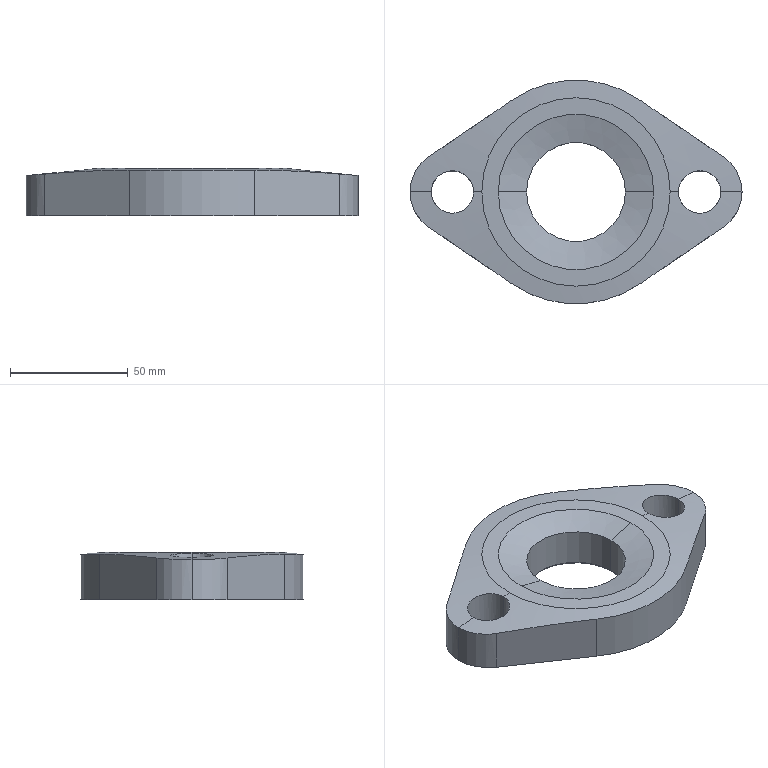Part | SolidWorks | features Chamfer 1, Extrusion 1, RevCut 1 | 1 solid | 23 faces | box 141 x 95 x 20 mm | volume 136049 mm3 | cylinder 11 | cone 6 | plane 6 | commonest cylinder face diameters 18 x4 36 x3 42 x2 95 x2
STEP:
#1=CARTESIAN_POINT('',(21.,0.,1.));
#2=VERTEX_POINT('',#1);
#3=CARTESIAN_POINT('',(-21.,0.,1.));
#4=VERTEX_POINT('',#3);
#5=CARTESIAN_POINT('',(0.,0.,1.));
#6=DIRECTION('',(0.,0.,-1.));
#7=DIRECTION('',(1.,0.,0.));
#8=AXIS2_PLACEMENT_3D('',#5,#6,#7);
#9=CIRCLE('',#8,21.);
#10=EDGE_CURVE('',#2,#4,#9,.T.);
#11=ORIENTED_EDGE('',*,*,#10,.F.);
#12=CARTESIAN_POINT('',(22.,0.,0.));
#13=VERTEX_POINT('',#12);
#14=CARTESIAN_POINT('',(21.,0.,1.));
#15=DIRECTION('',(0.7071,0.,-0.7071));
#16=VECTOR('',#15,1000.);
#17=LINE('',#14,#16);
#18=EDGE_CURVE('',#2,#13,#17,.T.);
#19=ORIENTED_EDGE('',*,*,#18,.T.);
#20=CARTESIAN_POINT('',(-22.,0.,0.));
#21=VERTEX_POINT('',#20);
#22=CARTESIAN_POINT('',(0.,0.,0.));
#23=DIRECTION('',(0.,0.,1.));
#24=DIRECTION('',(1.,0.,0.));
#25=AXIS2_PLACEMENT_3D('',#22,#23,#24);
#26=CIRCLE('',#25,22.);
#27=EDGE_CURVE('',#21,#13,#26,.T.);
#28=ORIENTED_EDGE('',*,*,#27,.F.);
#29=CARTESIAN_POINT('',(-21.,0.,1.));
#30=DIRECTION('',(-0.7071,0.,-0.7071));
#31=VECTOR('',#30,1000.);
#32=LINE('',#29,#31);
#33=EDGE_CURVE('',#4,#21,#32,.T.);
#34=ORIENTED_EDGE('',*,*,#33,.F.);
#35=EDGE_LOOP('',(#11,#19,#28,#34));
#36=FACE_OUTER_BOUND('',#35,.T.);
#37=CARTESIAN_POINT('',(0.,0.,1.));
#38=DIRECTION('',(0.,0.,-1.));
#39=DIRECTION('',(-1.,0.,0.));
#40=AXIS2_PLACEMENT_3D('',#37,#38,#39);
#41=CONICAL_SURFACE('',#40,21.,0.7854);
#42=ADVANCED_FACE('',(#36),#41,.F.);
#43=CARTESIAN_POINT('',(-40.,0.,20.));
#44=VERTEX_POINT('',#43);
#45=CARTESIAN_POINT('',(40.,0.,20.));
#46=VERTEX_POINT('',#45);
#47=CARTESIAN_POINT('',(0.,0.,20.));
#48=DIRECTION('',(0.,0.,-1.));
#49=DIRECTION('',(-1.,0.,0.));
#50=AXIS2_PLACEMENT_3D('',#47,#48,#49);
#51=CIRCLE('',#50,40.);
#52=EDGE_CURVE('',#44,#46,#51,.T.);
#53=ORIENTED_EDGE('',*,*,#52,.T.);
#54=CARTESIAN_POINT('',(43.5,0.,19.656));
#55=VERTEX_POINT('',#54);
#56=CARTESIAN_POINT('',(40.,0.,20.));
#57=DIRECTION('',(0.9952,0.,-0.09789));
#58=VECTOR('',#57,1000.);
#59=LINE('',#56,#58);
#60=EDGE_CURVE('',#46,#55,#59,.T.);
#61=ORIENTED_EDGE('',*,*,#60,.T.);
#62=CARTESIAN_POINT('',(61.5,0.,17.885));
#63=VERTEX_POINT('',#62);
#64=CARTESIAN_POINT('',(43.5,0.,19.656));
#65=CARTESIAN_POINT('',(43.5,0.5885,19.656));
#66=CARTESIAN_POINT('',(43.557,1.174,19.649));
#67=CARTESIAN_POINT('',(43.731,2.048,19.628));
#68=CARTESIAN_POINT('',(43.804,2.337,19.62));
#69=CARTESIAN_POINT('',(43.975,2.902,19.6));
#70=CARTESIAN_POINT('',(44.174,3.455,19.576));
#71=CARTESIAN_POINT('',(44.426,3.986,19.547));
#72=CARTESIAN_POINT('',(44.704,4.507,19.515));
#73=CARTESIAN_POINT('',(44.858,4.763,19.497));
#74=CARTESIAN_POINT('',(45.352,5.5,19.441));
#75=CARTESIAN_POINT('',(45.725,5.953,19.399));
#76=CARTESIAN_POINT('',(46.556,6.783,19.307));
#77=CARTESIAN_POINT('',(47.019,7.163,19.256));
#78=CARTESIAN_POINT('',(47.996,7.814,19.151));
#79=CARTESIAN_POINT('',(48.512,8.09,19.097));
#80=CARTESIAN_POINT('',(49.33,8.428,19.012));
#81=CARTESIAN_POINT('',(49.61,8.528,18.983));
#82=CARTESIAN_POINT('',(50.174,8.699,18.926));
#83=CARTESIAN_POINT('',(50.458,8.77,18.897));
#84=CARTESIAN_POINT('',(51.319,8.941,18.811));
#85=CARTESIAN_POINT('',(51.904,9.,18.753));
#86=CARTESIAN_POINT('',(53.089,9.,18.638));
#87=CARTESIAN_POINT('',(53.673,8.942,18.582));
#88=CARTESIAN_POINT('',(54.534,8.772,18.501));
#89=CARTESIAN_POINT('',(54.819,8.701,18.475));
#90=CARTESIAN_POINT('',(55.385,8.53,18.423));
#91=CARTESIAN_POINT('',(55.665,8.43,18.397));
#92=CARTESIAN_POINT('',(56.482,8.093,18.322));
#93=CARTESIAN_POINT('',(56.999,7.817,18.276));
#94=CARTESIAN_POINT('',(57.733,7.328,18.21));
#95=CARTESIAN_POINT('',(57.972,7.151,18.189));
#96=CARTESIAN_POINT('',(58.431,6.776,18.149));
#97=CARTESIAN_POINT('',(58.65,6.578,18.129));
#98=CARTESIAN_POINT('',(59.273,5.955,18.075));
#99=CARTESIAN_POINT('',(59.647,5.502,18.043));
#100=CARTESIAN_POINT('',(60.142,4.763,18.));
#101=CARTESIAN_POINT('',(60.296,4.507,17.987));
#102=CARTESIAN_POINT('',(60.574,3.987,17.963));
#103=CARTESIAN_POINT('',(60.826,3.456,17.942));
#104=CARTESIAN_POINT('',(61.024,2.902,17.925));
#105=CARTESIAN_POINT('',(61.196,2.337,17.911));
#106=CARTESIAN_POINT('',(61.269,2.047,17.905));
#107=CARTESIAN_POINT('',(61.443,1.174,17.89));
#108=CARTESIAN_POINT('',(61.5,0.5887,17.885));
#109=CARTESIAN_POINT('',(61.5,0.,17.885));
#110=B_SPLINE_CURVE_WITH_KNOTS('',3,(#64,#65,#66,#67,#68,#69,#70,#71,#72,#73,#74,#75,#76,#77,#78,#79,#80,#81,#82,#83,#84,#85,#86,#87,#88,#89,#90,#91,#92,#93,#94,#95,#96,#97,#98,#99,#100,#101,#102,#103,#104,#105,#106,#107,#108,#109),.UNSPECIFIED.,.F.,.F.,(4,2,2,1,2,2,2,2,2,2,2,2,2,2,2,2,2,2,2,2,1,2,2,4),(0.007109,0.008872,0.009754,0.01064,0.01152,0.0124,0.01416,0.01593,0.01769,0.01857,0.01945,0.02122,0.02298,0.02386,0.02474,0.02651,0.02739,0.02827,0.03003,0.03091,0.0318,0.03268,0.03356,0.03532),.UNSPECIFIED.);
#111=EDGE_CURVE('',#55,#63,#110,.T.);
#112=ORIENTED_EDGE('',*,*,#111,.T.);
#113=CARTESIAN_POINT('',(70.5,0.,17.));
#114=VERTEX_POINT('',#113);
#115=CARTESIAN_POINT('',(40.,0.,20.));
#116=DIRECTION('',(0.9952,0.,-0.09789));
#117=VECTOR('',#116,1000.);
#118=LINE('',#115,#117);
#119=EDGE_CURVE('',#63,#114,#118,.T.);
#120=ORIENTED_EDGE('',*,*,#119,.T.);
#121=CARTESIAN_POINT('',(62.614,14.89,17.604));
#122=VERTEX_POINT('',#121);
#123=CARTESIAN_POINT('',(62.614,14.89,17.604));
#124=CARTESIAN_POINT('',(63.833,14.062,17.506));
#125=CARTESIAN_POINT('',(64.927,13.103,17.421));
#126=CARTESIAN_POINT('',(66.144,11.746,17.327));
#127=CARTESIAN_POINT('',(66.38,11.467,17.309));
#128=CARTESIAN_POINT('',(66.835,10.892,17.274));
#129=CARTESIAN_POINT('',(67.056,10.595,17.257));
#130=CARTESIAN_POINT('',(67.686,9.691,17.209));
#131=CARTESIAN_POINT('',(68.066,9.068,17.181));
#132=CARTESIAN_POINT('',(68.747,7.783,17.13));
#133=CARTESIAN_POINT('',(69.048,7.12,17.107));
#134=CARTESIAN_POINT('',(69.571,5.754,17.068));
#135=CARTESIAN_POINT('',(69.794,5.046,17.052));
#136=CARTESIAN_POINT('',(70.323,2.913,17.013));
#137=CARTESIAN_POINT('',(70.5,1.468,17.));
#138=CARTESIAN_POINT('',(70.5,0.,17.));
#139=B_SPLINE_CURVE_WITH_KNOTS('',3,(#123,#124,#125,#126,#127,#128,#129,#130,#131,#132,#133,#134,#135,#136,#137,#138),.UNSPECIFIED.,.F.,.F.,(4,2,2,2,2,2,2,4),(0.000000239,0.004368,0.005459,0.006551,0.008735,0.01092,0.0131,0.01747),.UNSPECIFIED.);
#140=EDGE_CURVE('',#122,#114,#139,.T.);
#141=ORIENTED_EDGE('',*,*,#140,.F.);
#142=CARTESIAN_POINT('',(26.69,39.292,19.262));
#143=VERTEX_POINT('',#142);
#144=CARTESIAN_POINT('',(62.614,14.89,17.604));
#145=CARTESIAN_POINT('',(56.633,18.952,18.084));
#146=CARTESIAN_POINT('',(50.651,23.016,18.501));
#147=CARTESIAN_POINT('',(41.671,29.116,18.945));
#148=CARTESIAN_POINT('',(38.676,31.15,19.062));
#149=CARTESIAN_POINT('',(32.685,35.22,19.221));
#150=CARTESIAN_POINT('',(29.688,37.256,19.262));
#151=CARTESIAN_POINT('',(26.69,39.292,19.262));
#152=B_SPLINE_CURVE_WITH_KNOTS('',3,(#144,#145,#146,#147,#148,#149,#150,#151),.UNSPECIFIED.,.F.,.F.,(4,2,2,4),(0.000000242,0.02173,0.0326,0.04346),.UNSPECIFIED.);
#153=EDGE_CURVE('',#122,#143,#152,.T.);
#154=ORIENTED_EDGE('',*,*,#153,.T.);
#155=CARTESIAN_POINT('',(-26.69,39.292,19.262));
#156=VERTEX_POINT('',#155);
#157=CARTESIAN_POINT('',(0.,0.,19.262));
#158=DIRECTION('',(0.,0.,-1.));
#159=DIRECTION('',(-1.,0.,0.));
#160=AXIS2_PLACEMENT_3D('',#157,#158,#159);
#161=CIRCLE('',#160,47.5);
#162=EDGE_CURVE('',#156,#143,#161,.T.);
#163=ORIENTED_EDGE('',*,*,#162,.F.);
#164=CARTESIAN_POINT('',(-62.614,14.89,17.604));
#165=VERTEX_POINT('',#164);
#166=CARTESIAN_POINT('',(-62.614,14.89,17.604));
#167=CARTESIAN_POINT('',(-56.633,18.952,18.084));
#168=CARTESIAN_POINT('',(-50.651,23.016,18.501));
#169=CARTESIAN_POINT('',(-41.671,29.116,18.945));
#170=CARTESIAN_POINT('',(-38.676,31.15,19.062));
#171=CARTESIAN_POINT('',(-32.685,35.22,19.221));
#172=CARTESIAN_POINT('',(-29.688,37.256,19.262));
#173=CARTESIAN_POINT('',(-26.69,39.292,19.262));
#174=B_SPLINE_CURVE_WITH_KNOTS('',3,(#166,#167,#168,#169,#170,#171,#172,#173),.UNSPECIFIED.,.F.,.F.,(4,2,2,4),(0.000000242,0.02173,0.0326,0.04346),.UNSPECIFIED.);
#175=EDGE_CURVE('',#165,#156,#174,.T.);
#176=ORIENTED_EDGE('',*,*,#175,.F.);
#177=CARTESIAN_POINT('',(-70.5,0.,17.));
#178=VERTEX_POINT('',#177);
#179=CARTESIAN_POINT('',(-62.614,14.89,17.604));
#180=CARTESIAN_POINT('',(-63.833,14.062,17.506));
#181=CARTESIAN_POINT('',(-64.927,13.103,17.421));
#182=CARTESIAN_POINT('',(-66.144,11.746,17.327));
#183=CARTESIAN_POINT('',(-66.38,11.467,17.309));
#184=CARTESIAN_POINT('',(-66.835,10.892,17.274));
#185=CARTESIAN_POINT('',(-67.056,10.595,17.257));
#186=CARTESIAN_POINT('',(-67.686,9.691,17.209));
#187=CARTESIAN_POINT('',(-68.066,9.068,17.181));
#188=CARTESIAN_POINT('',(-68.747,7.783,17.13));
#189=CARTESIAN_POINT('',(-69.048,7.12,17.107));
#190=CARTESIAN_POINT('',(-69.571,5.754,17.068));
#191=CARTESIAN_POINT('',(-69.794,5.046,17.052));
#192=CARTESIAN_POINT('',(-70.323,2.913,17.013));
#193=CARTESIAN_POINT('',(-70.5,1.468,17.));
#194=CARTESIAN_POINT('',(-70.5,0.,17.));
#195=B_SPLINE_CURVE_WITH_KNOTS('',3,(#179,#180,#181,#182,#183,#184,#185,#186,#187,#188,#189,#190,#191,#192,#193,#194),.UNSPECIFIED.,.F.,.F.,(4,2,2,2,2,2,2,4),(0.000000239,0.004368,0.005459,0.006551,0.008735,0.01092,0.0131,0.01747),.UNSPECIFIED.);
#196=EDGE_CURVE('',#165,#178,#195,.T.);
#197=ORIENTED_EDGE('',*,*,#196,.T.);
#198=CARTESIAN_POINT('',(-61.5,0.,17.885));
#199=VERTEX_POINT('',#198);
#200=CARTESIAN_POINT('',(-40.,0.,20.));
#201=DIRECTION('',(-0.9952,0.,-0.09789));
#202=VECTOR('',#201,1000.);
#203=LINE('',#200,#202);
#204=EDGE_CURVE('',#199,#178,#203,.T.);
#205=ORIENTED_EDGE('',*,*,#204,.F.);
#206=CARTESIAN_POINT('',(-43.5,0.,19.656));
#207=VERTEX_POINT('',#206);
#208=CARTESIAN_POINT('',(-43.5,0.,19.656));
#209=CARTESIAN_POINT('',(-43.5,0.2974,19.656));
#210=CARTESIAN_POINT('',(-43.515,0.5945,19.654));
#211=CARTESIAN_POINT('',(-43.573,1.181,19.647));
#212=CARTESIAN_POINT('',(-43.66,1.763,19.637));
#213=CARTESIAN_POINT('',(-43.803,2.334,19.62));
#214=CARTESIAN_POINT('',(-43.975,2.899,19.6));
#215=CARTESIAN_POINT('',(-44.076,3.181,19.588));
#216=CARTESIAN_POINT('',(-44.416,4.,19.548));
#217=CARTESIAN_POINT('',(-44.694,4.517,19.516));
#218=CARTESIAN_POINT('',(-45.348,5.495,19.442));
#219=CARTESIAN_POINT('',(-45.729,5.958,19.399));
#220=CARTESIAN_POINT('',(-46.56,6.787,19.306));
#221=CARTESIAN_POINT('',(-47.013,7.158,19.257));
#222=CARTESIAN_POINT('',(-47.75,7.65,19.178));
#223=CARTESIAN_POINT('',(-48.005,7.803,19.151));
#224=CARTESIAN_POINT('',(-48.525,8.08,19.096));
#225=CARTESIAN_POINT('',(-49.055,8.33,19.04));
#226=CARTESIAN_POINT('',(-49.606,8.527,18.984));
#227=CARTESIAN_POINT('',(-50.167,8.697,18.926));
#228=CARTESIAN_POINT('',(-50.455,8.77,18.897));
#229=CARTESIAN_POINT('',(-51.325,8.943,18.81));
#230=CARTESIAN_POINT('',(-51.908,9.,18.753));
#231=CARTESIAN_POINT('',(-52.786,9.,18.667));
#232=CARTESIAN_POINT('',(-53.079,8.986,18.639));
#233=CARTESIAN_POINT('',(-53.667,8.929,18.583));
#234=CARTESIAN_POINT('',(-53.962,8.885,18.555));
#235=CARTESIAN_POINT('',(-54.827,8.714,18.474));
#236=CARTESIAN_POINT('',(-55.387,8.545,18.422));
#237=CARTESIAN_POINT('',(-56.202,8.208,18.348));
#238=CARTESIAN_POINT('',(-56.472,8.082,18.323));
#239=CARTESIAN_POINT('',(-56.994,7.803,18.276));
#240=CARTESIAN_POINT('',(-57.246,7.652,18.254));
#241=CARTESIAN_POINT('',(-57.978,7.165,18.188));
#242=CARTESIAN_POINT('',(-58.433,6.793,18.148));
#243=CARTESIAN_POINT('',(-59.063,6.165,18.093));
#244=CARTESIAN_POINT('',(-59.263,5.945,18.076));
#245=CARTESIAN_POINT('',(-59.637,5.49,18.044));
#246=CARTESIAN_POINT('',(-59.988,5.019,18.014));
#247=CARTESIAN_POINT('',(-60.291,4.515,17.988));
#248=CARTESIAN_POINT('',(-60.57,3.995,17.964));
#249=CARTESIAN_POINT('',(-60.698,3.725,17.953));
#250=CARTESIAN_POINT('',(-61.039,2.904,17.924));
#251=CARTESIAN_POINT('',(-61.21,2.342,17.91));
#252=CARTESIAN_POINT('',(-61.441,1.187,17.89));
#253=CARTESIAN_POINT('',(-61.5,0.5893,17.885));
#254=CARTESIAN_POINT('',(-61.5,0.,17.885));
#255=B_SPLINE_CURVE_WITH_KNOTS('',3,(#208,#209,#210,#211,#212,#213,#214,#215,#216,#217,#218,#219,#220,#221,#222,#223,#224,#225,#226,#227,#228,#229,#230,#231,#232,#233,#234,#235,#236,#237,#238,#239,#240,#241,#242,#243,#244,#245,#246,#247,#248,#249,#250,#251,#252,#253,#254),.UNSPECIFIED.,.F.,.F.,(4,2,1,2,2,2,2,2,2,1,2,2,2,2,2,2,2,2,2,2,1,2,2,2,4),(0.02115,0.02203,0.02291,0.02379,0.02467,0.02643,0.0282,0.02996,0.03084,0.03172,0.0326,0.03349,0.03525,0.03613,0.03701,0.03877,0.03965,0.04054,0.0423,0.04318,0.04406,0.04494,0.04582,0.04759,0.04935),.UNSPECIFIED.);
#256=EDGE_CURVE('',#207,#199,#255,.T.);
#257=ORIENTED_EDGE('',*,*,#256,.F.);
#258=CARTESIAN_POINT('',(-40.,0.,20.));
#259=DIRECTION('',(-0.9952,0.,-0.09789));
#260=VECTOR('',#259,1000.);
#261=LINE('',#258,#260);
#262=EDGE_CURVE('',#44,#207,#261,.T.);
#263=ORIENTED_EDGE('',*,*,#262,.F.);
#264=EDGE_LOOP('',(#53,#61,#112,#120,#141,#154,#163,#176,#197,#205,#257,#263));
#265=FACE_OUTER_BOUND('',#264,.T.);
#266=CARTESIAN_POINT('',(0.,0.,20.));
#267=DIRECTION('',(0.,0.,-1.));
#268=DIRECTION('',(-1.,0.,0.));
#269=AXIS2_PLACEMENT_3D('',#266,#267,#268);
#270=CONICAL_SURFACE('',#269,40.,1.473);
#271=ADVANCED_FACE('',(#265),#270,.T.);
#272=CARTESIAN_POINT('',(21.,0.,16.785));
#273=VERTEX_POINT('',#272);
#274=CARTESIAN_POINT('',(-21.,0.,16.785));
#275=VERTEX_POINT('',#274);
#276=CARTESIAN_POINT('',(0.,0.,16.785));
#277=DIRECTION('',(0.,0.,-1.));
#278=DIRECTION('',(-1.,0.,0.));
#279=AXIS2_PLACEMENT_3D('',#276,#277,#278);
#280=CIRCLE('',#279,21.);
#281=EDGE_CURVE('',#273,#275,#280,.T.);
#282=ORIENTED_EDGE('',*,*,#281,.T.);
#283=CARTESIAN_POINT('',(-33.,0.,20.));
#284=VERTEX_POINT('',#283);
#285=CARTESIAN_POINT('',(-21.,0.,16.785));
#286=DIRECTION('',(-0.9659,0.,0.2588));
#287=VECTOR('',#286,1000.);
#288=LINE('',#285,#287);
#289=EDGE_CURVE('',#275,#284,#288,.T.);
#290=ORIENTED_EDGE('',*,*,#289,.T.);
#291=CARTESIAN_POINT('',(33.,0.,20.));
#292=VERTEX_POINT('',#291);
#293=CARTESIAN_POINT('',(0.,0.,20.));
#294=DIRECTION('',(0.,0.,-1.));
#295=DIRECTION('',(-1.,0.,0.));
#296=AXIS2_PLACEMENT_3D('',#293,#294,#295);
#297=CIRCLE('',#296,33.);
#298=EDGE_CURVE('',#292,#284,#297,.T.);
#299=ORIENTED_EDGE('',*,*,#298,.F.);
#300=CARTESIAN_POINT('',(21.,0.,16.785));
#301=DIRECTION('',(0.9659,0.,0.2588));
#302=VECTOR('',#301,1000.);
#303=LINE('',#300,#302);
#304=EDGE_CURVE('',#273,#292,#303,.T.);
#305=ORIENTED_EDGE('',*,*,#304,.F.);
#306=EDGE_LOOP('',(#282,#290,#299,#305));
#307=FACE_OUTER_BOUND('',#306,.T.);
#308=CARTESIAN_POINT('',(0.,0.,16.785));
#309=DIRECTION('',(0.,0.,1.));
#310=DIRECTION('',(1.,0.,0.));
#311=AXIS2_PLACEMENT_3D('',#308,#309,#310);
#312=CONICAL_SURFACE('',#311,21.,1.309);
#313=ADVANCED_FACE('',(#307),#312,.F.);
#314=ORIENTED_EDGE('',*,*,#281,.F.);
#315=CARTESIAN_POINT('',(21.,0.,0.));
#316=DIRECTION('',(0.,0.,-1.));
#317=VECTOR('',#316,1000.);
#318=LINE('',#315,#317);
#319=EDGE_CURVE('',#273,#2,#318,.T.);
#320=ORIENTED_EDGE('',*,*,#319,.T.);
#321=ORIENTED_EDGE('',*,*,#10,.T.);
#322=CARTESIAN_POINT('',(-21.,0.,0.));
#323=DIRECTION('',(0.,0.,-1.));
#324=VECTOR('',#323,1000.);
#325=LINE('',#322,#324);
#326=EDGE_CURVE('',#275,#4,#325,.T.);
#327=ORIENTED_EDGE('',*,*,#326,.F.);
#328=EDGE_LOOP('',(#314,#320,#321,#327));
#329=FACE_OUTER_BOUND('',#328,.T.);
#330=CARTESIAN_POINT('',(0.,0.,0.));
#331=DIRECTION('',(0.,0.,-1.));
#332=DIRECTION('',(-1.,0.,0.));
#333=AXIS2_PLACEMENT_3D('',#330,#331,#332);
#334=CYLINDRICAL_SURFACE('',#333,21.);
#335=ADVANCED_FACE('',(#329),#334,.F.);
#336=CARTESIAN_POINT('',(-61.5,0.,17.885));
#337=CARTESIAN_POINT('',(-61.5,-0.5893,17.885));
#338=CARTESIAN_POINT('',(-61.443,-1.174,17.89));
#339=CARTESIAN_POINT('',(-61.27,-2.045,17.905));
#340=CARTESIAN_POINT('',(-61.197,-2.335,17.911));
#341=CARTESIAN_POINT('',(-61.025,-2.901,17.925));
#342=CARTESIAN_POINT('',(-60.925,-3.178,17.934));
#343=CARTESIAN_POINT('',(-60.588,-3.992,17.962));
#344=CARTESIAN_POINT('',(-60.31,-4.513,17.986));
#345=CARTESIAN_POINT('',(-59.648,-5.501,18.043));
#346=CARTESIAN_POINT('',(-59.272,-5.958,18.075));
#347=CARTESIAN_POINT('',(-58.429,-6.797,18.149));
#348=CARTESIAN_POINT('',(-57.973,-7.169,18.189));
#349=CARTESIAN_POINT('',(-57.241,-7.656,18.254));
#350=CARTESIAN_POINT('',(-56.989,-7.806,18.277));
#351=CARTESIAN_POINT('',(-56.468,-8.083,18.324));
#352=CARTESIAN_POINT('',(-56.198,-8.21,18.348));
#353=CARTESIAN_POINT('',(-55.381,-8.547,18.423));
#354=CARTESIAN_POINT('',(-54.82,-8.716,18.475));
#355=CARTESIAN_POINT('',(-53.669,-8.943,18.583));
#356=CARTESIAN_POINT('',(-53.073,-9.001,18.64));
#357=CARTESIAN_POINT('',(-51.902,-8.999,18.753));
#358=CARTESIAN_POINT('',(-51.319,-8.942,18.811));
#359=CARTESIAN_POINT('',(-50.451,-8.769,18.898));
#360=CARTESIAN_POINT('',(-50.163,-8.696,18.927));
#361=CARTESIAN_POINT('',(-49.6,-8.525,18.984));
#362=CARTESIAN_POINT('',(-49.049,-8.328,19.041));
#363=CARTESIAN_POINT('',(-48.52,-8.077,19.096));
#364=CARTESIAN_POINT('',(-48.002,-7.801,19.151));
#365=CARTESIAN_POINT('',(-47.747,-7.648,19.178));
#366=CARTESIAN_POINT('',(-47.009,-7.155,19.257));
#367=CARTESIAN_POINT('',(-46.556,-6.783,19.307));
#368=CARTESIAN_POINT('',(-45.934,-6.162,19.376));
#369=CARTESIAN_POINT('',(-45.736,-5.944,19.398));
#370=CARTESIAN_POINT('',(-45.36,-5.487,19.44));
#371=CARTESIAN_POINT('',(-45.182,-5.248,19.46));
#372=CARTESIAN_POINT('',(-44.691,-4.513,19.516));
#373=CARTESIAN_POINT('',(-44.414,-3.996,19.548));
#374=CARTESIAN_POINT('',(-44.075,-3.179,19.588));
#375=CARTESIAN_POINT('',(-43.974,-2.898,19.6));
#376=CARTESIAN_POINT('',(-43.802,-2.331,19.62));
#377=CARTESIAN_POINT('',(-43.73,-2.045,19.628));
#378=CARTESIAN_POINT('',(-43.558,-1.18,19.649));
#379=CARTESIAN_POINT('',(-43.5,-0.5947,19.656));
#380=CARTESIAN_POINT('',(-43.5,0.,19.656));
#381=B_SPLINE_CURVE_WITH_KNOTS('',3,(#336,#337,#338,#339,#340,#341,#342,#343,#344,#345,#346,#347,#348,#349,#350,#351,#352,#353,#354,#355,#356,#357,#358,#359,#360,#361,#362,#363,#364,#365,#366,#367,#368,#369,#370,#371,#372,#373,#374,#375,#376,#377,#378,#379,#380),.UNSPECIFIED.,.F.,.F.,(4,2,2,2,2,2,2,2,2,2,2,2,2,1,2,2,2,2,2,2,2,2,4),(0.04935,0.05111,0.05199,0.05287,0.05464,0.0564,0.05816,0.05904,0.05992,0.06169,0.06345,0.06521,0.06609,0.06697,0.06786,0.06874,0.0705,0.07138,0.07226,0.07402,0.07491,0.07579,0.07755),.UNSPECIFIED.);
#382=EDGE_CURVE('',#199,#207,#381,.T.);
#383=ORIENTED_EDGE('',*,*,#382,.T.);
#384=CARTESIAN_POINT('',(-43.5,0.,0.));
#385=VERTEX_POINT('',#384);
#386=CARTESIAN_POINT('',(-43.5,0.,20.));
#387=DIRECTION('',(0.,0.,-1.));
#388=VECTOR('',#387,1000.);
#389=LINE('',#386,#388);
#390=EDGE_CURVE('',#207,#385,#389,.T.);
#391=ORIENTED_EDGE('',*,*,#390,.T.);
#392=CARTESIAN_POINT('',(-61.5,0.,0.));
#393=VERTEX_POINT('',#392);
#394=CARTESIAN_POINT('',(-52.5,0.,0.));
#395=DIRECTION('',(0.,0.,-1.));
#396=DIRECTION('',(1.,0.,0.));
#397=AXIS2_PLACEMENT_3D('',#394,#395,#396);
#398=CIRCLE('',#397,9.);
#399=EDGE_CURVE('',#385,#393,#398,.T.);
#400=ORIENTED_EDGE('',*,*,#399,.T.);
#401=CARTESIAN_POINT('',(-61.5,0.,20.));
#402=DIRECTION('',(0.,0.,-1.));
#403=VECTOR('',#402,1000.);
#404=LINE('',#401,#403);
#405=EDGE_CURVE('',#199,#393,#404,.T.);
#406=ORIENTED_EDGE('',*,*,#405,.F.);
#407=EDGE_LOOP('',(#383,#391,#400,#406));
#408=FACE_OUTER_BOUND('',#407,.T.);
#409=CARTESIAN_POINT('',(-52.5,0.,20.));
#410=DIRECTION('',(0.,0.,-1.));
#411=DIRECTION('',(-1.,0.,0.));
#412=AXIS2_PLACEMENT_3D('',#409,#410,#411);
#413=CYLINDRICAL_SURFACE('',#412,9.);
#414=ADVANCED_FACE('',(#408),#413,.F.);
#415=CARTESIAN_POINT('',(-62.614,-14.89,17.604));
#416=VERTEX_POINT('',#415);
#417=CARTESIAN_POINT('',(-70.5,0.,17.));
#418=CARTESIAN_POINT('',(-70.5,-0.3665,17.));
#419=CARTESIAN_POINT('',(-70.489,-0.7358,17.001));
#420=CARTESIAN_POINT('',(-70.444,-1.469,17.004));
#421=CARTESIAN_POINT('',(-70.41,-1.833,17.007));
#422=CARTESIAN_POINT('',(-70.277,-2.919,17.016));
#423=CARTESIAN_POINT('',(-70.144,-3.634,17.026));
#424=CARTESIAN_POINT('',(-69.794,-5.045,17.052));
#425=CARTESIAN_POINT('',(-69.576,-5.742,17.068));
#426=CARTESIAN_POINT('',(-69.05,-7.117,17.107));
#427=CARTESIAN_POINT('',(-68.746,-7.784,17.13));
#428=CARTESIAN_POINT('',(-68.065,-9.07,17.181));
#429=CARTESIAN_POINT('',(-67.687,-9.69,17.209));
#430=CARTESIAN_POINT('',(-67.063,-10.585,17.256));
#431=CARTESIAN_POINT('',(-66.846,-10.878,17.273));
#432=CARTESIAN_POINT('',(-66.392,-11.452,17.308));
#433=CARTESIAN_POINT('',(-66.154,-11.734,17.326));
#434=CARTESIAN_POINT('',(-64.929,-13.102,17.42));
#435=CARTESIAN_POINT('',(-63.831,-14.063,17.506));
#436=CARTESIAN_POINT('',(-62.614,-14.89,17.604));
#437=B_SPLINE_CURVE_WITH_KNOTS('',3,(#417,#418,#419,#420,#421,#422,#423,#424,#425,#426,#427,#428,#429,#430,#431,#432,#433,#434,#435,#436),.UNSPECIFIED.,.F.,.F.,(4,2,2,2,2,2,2,2,2,4),(0.01747,0.01856,0.01965,0.02183,0.02401,0.02619,0.02837,0.02946,0.03055,0.03491),.UNSPECIFIED.);
#438=EDGE_CURVE('',#178,#416,#437,.T.);
#439=ORIENTED_EDGE('',*,*,#438,.F.);
#440=CARTESIAN_POINT('',(-70.5,0.,0.));
#441=VERTEX_POINT('',#440);
#442=CARTESIAN_POINT('',(-70.5,0.,20.));
#443=DIRECTION('',(0.,0.,-1.));
#444=VECTOR('',#443,1000.);
#445=LINE('',#442,#444);
#446=EDGE_CURVE('',#178,#441,#445,.T.);
#447=ORIENTED_EDGE('',*,*,#446,.T.);
#448=CARTESIAN_POINT('',(-62.614,-14.89,0.));
#449=VERTEX_POINT('',#448);
#450=CARTESIAN_POINT('',(-52.5,0.,0.));
#451=DIRECTION('',(0.,0.,-1.));
#452=DIRECTION('',(1.,0.,0.));
#453=AXIS2_PLACEMENT_3D('',#450,#451,#452);
#454=CIRCLE('',#453,18.);
#455=EDGE_CURVE('',#449,#441,#454,.T.);
#456=ORIENTED_EDGE('',*,*,#455,.F.);
#457=CARTESIAN_POINT('',(-62.614,-14.89,20.));
#458=DIRECTION('',(0.,0.,-1.));
#459=VECTOR('',#458,1000.);
#460=LINE('',#457,#459);
#461=EDGE_CURVE('',#416,#449,#460,.T.);
#462=ORIENTED_EDGE('',*,*,#461,.F.);
#463=EDGE_LOOP('',(#439,#447,#456,#462));
#464=FACE_OUTER_BOUND('',#463,.T.);
#465=CARTESIAN_POINT('',(-52.5,0.,20.));
#466=DIRECTION('',(0.,0.,-1.));
#467=DIRECTION('',(-1.,0.,0.));
#468=AXIS2_PLACEMENT_3D('',#465,#466,#467);
#469=CYLINDRICAL_SURFACE('',#468,18.);
#470=ADVANCED_FACE('',(#464),#469,.T.);
#471=CARTESIAN_POINT('',(61.5,0.,17.885));
#472=CARTESIAN_POINT('',(61.5,-0.5883,17.885));
#473=CARTESIAN_POINT('',(61.441,-1.186,17.89));
#474=CARTESIAN_POINT('',(61.21,-2.342,17.91));
#475=CARTESIAN_POINT('',(61.039,-2.904,17.924));
#476=CARTESIAN_POINT('',(60.699,-3.722,17.953));
#477=CARTESIAN_POINT('',(60.571,-3.992,17.964));
#478=CARTESIAN_POINT('',(60.292,-4.514,17.988));
#479=CARTESIAN_POINT('',(60.14,-4.766,18.));
#480=CARTESIAN_POINT('',(59.65,-5.497,18.043));
#481=CARTESIAN_POINT('',(59.277,-5.952,18.075));
#482=CARTESIAN_POINT('',(58.435,-6.792,18.148));
#483=CARTESIAN_POINT('',(57.98,-7.163,18.188));
#484=CARTESIAN_POINT('',(57.249,-7.651,18.253));
#485=CARTESIAN_POINT('',(56.997,-7.802,18.276));
#486=CARTESIAN_POINT('',(56.476,-8.08,18.323));
#487=CARTESIAN_POINT('',(56.206,-8.207,18.347));
#488=CARTESIAN_POINT('',(55.39,-8.544,18.422));
#489=CARTESIAN_POINT('',(54.83,-8.713,18.474));
#490=CARTESIAN_POINT('',(53.966,-8.885,18.555));
#491=CARTESIAN_POINT('',(53.673,-8.928,18.583));
#492=CARTESIAN_POINT('',(53.084,-8.986,18.639));
#493=CARTESIAN_POINT('',(52.791,-9.,18.667));
#494=CARTESIAN_POINT('',(51.912,-9.,18.752));
#495=CARTESIAN_POINT('',(51.33,-8.943,18.81));
#496=CARTESIAN_POINT('',(50.462,-8.771,18.897));
#497=CARTESIAN_POINT('',(50.173,-8.699,18.926));
#498=CARTESIAN_POINT('',(49.611,-8.529,18.983));
#499=CARTESIAN_POINT('',(49.06,-8.332,19.04));
#500=CARTESIAN_POINT('',(48.53,-8.083,19.095));
#501=CARTESIAN_POINT('',(48.012,-7.807,19.15));
#502=CARTESIAN_POINT('',(47.757,-7.655,19.177));
#503=CARTESIAN_POINT('',(47.018,-7.162,19.256));
#504=CARTESIAN_POINT('',(46.56,-6.788,19.306));
#505=CARTESIAN_POINT('',(45.721,-5.949,19.4));
#506=CARTESIAN_POINT('',(45.348,-5.495,19.442));
#507=CARTESIAN_POINT('',(44.859,-4.764,19.497));
#508=CARTESIAN_POINT('',(44.707,-4.512,19.515));
#509=CARTESIAN_POINT('',(44.428,-3.991,19.547));
#510=CARTESIAN_POINT('',(44.3,-3.721,19.562));
#511=CARTESIAN_POINT('',(43.961,-2.903,19.601));
#512=CARTESIAN_POINT('',(43.79,-2.342,19.621));
#513=CARTESIAN_POINT('',(43.617,-1.474,19.642));
#514=CARTESIAN_POINT('',(43.573,-1.18,19.647));
#515=CARTESIAN_POINT('',(43.514,-0.5888,19.654));
#516=CARTESIAN_POINT('',(43.5,-0.294,19.656));
#517=CARTESIAN_POINT('',(43.5,0.,19.656));
#518=B_SPLINE_CURVE_WITH_KNOTS('',3,(#471,#472,#473,#474,#475,#476,#477,#478,#479,#480,#481,#482,#483,#484,#485,#486,#487,#488,#489,#490,#491,#492,#493,#494,#495,#496,#497,#498,#499,#500,#501,#502,#503,#504,#505,#506,#507,#508,#509,#510,#511,#512,#513,#514,#515,#516,#517),.UNSPECIFIED.,.F.,.F.,(4,2,2,2,2,2,2,2,2,2,2,2,2,2,1,2,2,2,2,2,2,2,2,4),(0.03532,0.03708,0.03885,0.03973,0.04061,0.04237,0.04413,0.04501,0.0459,0.04766,0.04854,0.04942,0.05118,0.05206,0.05294,0.05383,0.05471,0.05647,0.05823,0.05911,0.05999,0.06175,0.06264,0.06352),.UNSPECIFIED.);
#519=EDGE_CURVE('',#63,#55,#518,.T.);
#520=ORIENTED_EDGE('',*,*,#519,.F.);
#521=CARTESIAN_POINT('',(61.5,0.,0.));
#522=VERTEX_POINT('',#521);
#523=CARTESIAN_POINT('',(61.5,0.,20.));
#524=DIRECTION('',(0.,0.,-1.));
#525=VECTOR('',#524,1000.);
#526=LINE('',#523,#525);
#527=EDGE_CURVE('',#63,#522,#526,.T.);
#528=ORIENTED_EDGE('',*,*,#527,.T.);
#529=CARTESIAN_POINT('',(43.5,0.,0.));
#530=VERTEX_POINT('',#529);
#531=CARTESIAN_POINT('',(52.5,0.,0.));
#532=DIRECTION('',(0.,0.,1.));
#533=DIRECTION('',(1.,0.,0.));
#534=AXIS2_PLACEMENT_3D('',#531,#532,#533);
#535=CIRCLE('',#534,9.);
#536=EDGE_CURVE('',#530,#522,#535,.T.);
#537=ORIENTED_EDGE('',*,*,#536,.F.);
#538=CARTESIAN_POINT('',(43.5,0.,20.));
#539=DIRECTION('',(0.,0.,-1.));
#540=VECTOR('',#539,1000.);
#541=LINE('',#538,#540);
#542=EDGE_CURVE('',#55,#530,#541,.T.);
#543=ORIENTED_EDGE('',*,*,#542,.F.);
#544=EDGE_LOOP('',(#520,#528,#537,#543));
#545=FACE_OUTER_BOUND('',#544,.T.);
#546=CARTESIAN_POINT('',(52.5,0.,20.));
#547=DIRECTION('',(0.,0.,-1.));
#548=DIRECTION('',(-1.,0.,0.));
#549=AXIS2_PLACEMENT_3D('',#546,#547,#548);
#550=CYLINDRICAL_SURFACE('',#549,9.);
#551=ADVANCED_FACE('',(#545),#550,.F.);
#552=CARTESIAN_POINT('',(-26.69,-39.292,19.262));
#553=VERTEX_POINT('',#552);
#554=CARTESIAN_POINT('',(-62.614,-14.89,17.604));
#555=CARTESIAN_POINT('',(-56.633,-18.952,18.084));
#556=CARTESIAN_POINT('',(-50.651,-23.016,18.501));
#557=CARTESIAN_POINT('',(-41.671,-29.116,18.945));
#558=CARTESIAN_POINT('',(-38.676,-31.15,19.062));
#559=CARTESIAN_POINT('',(-32.685,-35.22,19.221));
#560=CARTESIAN_POINT('',(-29.688,-37.256,19.262));
#561=CARTESIAN_POINT('',(-26.69,-39.292,19.262));
#562=B_SPLINE_CURVE_WITH_KNOTS('',3,(#554,#555,#556,#557,#558,#559,#560,#561),.UNSPECIFIED.,.F.,.F.,(4,2,2,4),(0.000000242,0.02173,0.0326,0.04346),.UNSPECIFIED.);
#563=EDGE_CURVE('',#416,#553,#562,.T.);
#564=ORIENTED_EDGE('',*,*,#563,.F.);
#565=ORIENTED_EDGE('',*,*,#461,.T.);
#566=CARTESIAN_POINT('',(-26.69,-39.292,0.));
#567=VERTEX_POINT('',#566);
#568=CARTESIAN_POINT('',(-26.69,-39.292,0.));
#569=DIRECTION('',(-0.8272,0.5619,0.));
#570=VECTOR('',#569,1000.);
#571=LINE('',#568,#570);
#572=EDGE_CURVE('',#567,#449,#571,.T.);
#573=ORIENTED_EDGE('',*,*,#572,.F.);
#574=CARTESIAN_POINT('',(-26.69,-39.292,20.));
#575=DIRECTION('',(0.,0.,-1.));
#576=VECTOR('',#575,1000.);
#577=LINE('',#574,#576);
#578=EDGE_CURVE('',#553,#567,#577,.T.);
#579=ORIENTED_EDGE('',*,*,#578,.F.);
#580=EDGE_LOOP('',(#564,#565,#573,#579));
#581=FACE_OUTER_BOUND('',#580,.T.);
#582=CARTESIAN_POINT('',(-26.69,-39.292,20.));
#583=DIRECTION('',(-0.5619,-0.8272,0.));
#584=DIRECTION('',(0.8272,-0.5619,0.));
#585=AXIS2_PLACEMENT_3D('',#582,#583,#584);
#586=PLANE('',#585);
#587=ADVANCED_FACE('',(#581),#586,.T.);
#588=CARTESIAN_POINT('',(26.69,-39.292,19.262));
#589=VERTEX_POINT('',#588);
#590=CARTESIAN_POINT('',(0.,0.,19.262));
#591=DIRECTION('',(0.,0.,1.));
#592=DIRECTION('',(-1.,0.,0.));
#593=AXIS2_PLACEMENT_3D('',#590,#591,#592);
#594=CIRCLE('',#593,47.5);
#595=EDGE_CURVE('',#553,#589,#594,.T.);
#596=ORIENTED_EDGE('',*,*,#595,.F.);
#597=ORIENTED_EDGE('',*,*,#578,.T.);
#598=CARTESIAN_POINT('',(26.69,-39.292,0.));
#599=VERTEX_POINT('',#598);
#600=CARTESIAN_POINT('',(0.,0.,0.));
#601=DIRECTION('',(0.,0.,-1.));
#602=DIRECTION('',(1.,0.,0.));
#603=AXIS2_PLACEMENT_3D('',#600,#601,#602);
#604=CIRCLE('',#603,47.5);
#605=EDGE_CURVE('',#599,#567,#604,.T.);
#606=ORIENTED_EDGE('',*,*,#605,.F.);
#607=CARTESIAN_POINT('',(26.69,-39.292,20.));
#608=DIRECTION('',(0.,0.,-1.));
#609=VECTOR('',#608,1000.);
#610=LINE('',#607,#609);
#611=EDGE_CURVE('',#589,#599,#610,.T.);
#612=ORIENTED_EDGE('',*,*,#611,.F.);
#613=EDGE_LOOP('',(#596,#597,#606,#612));
#614=FACE_OUTER_BOUND('',#613,.T.);
#615=CARTESIAN_POINT('',(0.,0.,20.));
#616=DIRECTION('',(0.,0.,-1.));
#617=DIRECTION('',(-1.,0.,0.));
#618=AXIS2_PLACEMENT_3D('',#615,#616,#617);
#619=CYLINDRICAL_SURFACE('',#618,47.5);
#620=ADVANCED_FACE('',(#614),#619,.T.);
#621=CARTESIAN_POINT('',(62.614,-14.89,17.604));
#622=VERTEX_POINT('',#621);
#623=CARTESIAN_POINT('',(62.614,-14.89,0.));
#624=VERTEX_POINT('',#623);
#625=CARTESIAN_POINT('',(62.614,-14.89,20.));
#626=DIRECTION('',(0.,0.,-1.));
#627=VECTOR('',#626,1000.);
#628=LINE('',#625,#627);
#629=EDGE_CURVE('',#622,#624,#628,.T.);
#630=ORIENTED_EDGE('',*,*,#629,.F.);
#631=CARTESIAN_POINT('',(62.614,-14.89,17.604));
#632=CARTESIAN_POINT('',(56.633,-18.952,18.084));
#633=CARTESIAN_POINT('',(50.651,-23.016,18.501));
#634=CARTESIAN_POINT('',(41.671,-29.116,18.945));
#635=CARTESIAN_POINT('',(38.676,-31.15,19.062));
#636=CARTESIAN_POINT('',(32.685,-35.22,19.221));
#637=CARTESIAN_POINT('',(29.688,-37.256,19.262));
#638=CARTESIAN_POINT('',(26.69,-39.292,19.262));
#639=B_SPLINE_CURVE_WITH_KNOTS('',3,(#631,#632,#633,#634,#635,#636,#637,#638),.UNSPECIFIED.,.F.,.F.,(4,2,2,4),(0.000000242,0.02173,0.0326,0.04346),.UNSPECIFIED.);
#640=EDGE_CURVE('',#622,#589,#639,.T.);
#641=ORIENTED_EDGE('',*,*,#640,.T.);
#642=ORIENTED_EDGE('',*,*,#611,.T.);
#643=CARTESIAN_POINT('',(26.69,-39.292,0.));
#644=DIRECTION('',(0.8272,0.5619,0.));
#645=VECTOR('',#644,1000.);
#646=LINE('',#643,#645);
#647=EDGE_CURVE('',#599,#624,#646,.T.);
#648=ORIENTED_EDGE('',*,*,#647,.T.);
#649=EDGE_LOOP('',(#630,#641,#642,#648));
#650=FACE_OUTER_BOUND('',#649,.T.);
#651=CARTESIAN_POINT('',(26.69,-39.292,20.));
#652=DIRECTION('',(-0.5619,0.8272,0.));
#653=DIRECTION('',(-0.8272,-0.5619,0.));
#654=AXIS2_PLACEMENT_3D('',#651,#652,#653);
#655=PLANE('',#654);
#656=ADVANCED_FACE('',(#650),#655,.F.);
#657=CARTESIAN_POINT('',(62.614,14.89,0.));
#658=VERTEX_POINT('',#657);
#659=CARTESIAN_POINT('',(62.614,14.89,20.));
#660=DIRECTION('',(0.,0.,-1.));
#661=VECTOR('',#660,1000.);
#662=LINE('',#659,#661);
#663=EDGE_CURVE('',#122,#658,#662,.T.);
#664=ORIENTED_EDGE('',*,*,#663,.F.);
#665=ORIENTED_EDGE('',*,*,#140,.T.);
#666=CARTESIAN_POINT('',(70.5,0.,17.));
#667=CARTESIAN_POINT('',(70.5,-0.3665,17.));
#668=CARTESIAN_POINT('',(70.489,-0.7358,17.001));
#669=CARTESIAN_POINT('',(70.444,-1.469,17.004));
#670=CARTESIAN_POINT('',(70.41,-1.833,17.007));
#671=CARTESIAN_POINT('',(70.277,-2.919,17.016));
#672=CARTESIAN_POINT('',(70.144,-3.634,17.026));
#673=CARTESIAN_POINT('',(69.794,-5.045,17.052));
#674=CARTESIAN_POINT('',(69.576,-5.742,17.068));
#675=CARTESIAN_POINT('',(69.05,-7.117,17.107));
#676=CARTESIAN_POINT('',(68.746,-7.784,17.13));
#677=CARTESIAN_POINT('',(68.065,-9.07,17.181));
#678=CARTESIAN_POINT('',(67.687,-9.69,17.209));
#679=CARTESIAN_POINT('',(67.063,-10.585,17.256));
#680=CARTESIAN_POINT('',(66.846,-10.878,17.273));
#681=CARTESIAN_POINT('',(66.392,-11.452,17.308));
#682=CARTESIAN_POINT('',(66.154,-11.734,17.326));
#683=CARTESIAN_POINT('',(64.929,-13.102,17.42));
#684=CARTESIAN_POINT('',(63.831,-14.063,17.506));
#685=CARTESIAN_POINT('',(62.614,-14.89,17.604));
#686=B_SPLINE_CURVE_WITH_KNOTS('',3,(#666,#667,#668,#669,#670,#671,#672,#673,#674,#675,#676,#677,#678,#679,#680,#681,#682,#683,#684,#685),.UNSPECIFIED.,.F.,.F.,(4,2,2,2,2,2,2,2,2,4),(0.01747,0.01856,0.01965,0.02183,0.02401,0.02619,0.02837,0.02946,0.03055,0.03491),.UNSPECIFIED.);
#687=EDGE_CURVE('',#114,#622,#686,.T.);
#688=ORIENTED_EDGE('',*,*,#687,.T.);
#689=ORIENTED_EDGE('',*,*,#629,.T.);
#690=CARTESIAN_POINT('',(52.5,0.,0.));
#691=DIRECTION('',(0.,0.,1.));
#692=DIRECTION('',(1.,0.,0.));
#693=AXIS2_PLACEMENT_3D('',#690,#691,#692);
#694=CIRCLE('',#693,18.);
#695=EDGE_CURVE('',#624,#658,#694,.T.);
#696=ORIENTED_EDGE('',*,*,#695,.T.);
#697=EDGE_LOOP('',(#664,#665,#688,#689,#696));
#698=FACE_OUTER_BOUND('',#697,.T.);
#699=CARTESIAN_POINT('',(52.5,0.,20.));
#700=DIRECTION('',(0.,0.,-1.));
#701=DIRECTION('',(-1.,0.,0.));
#702=AXIS2_PLACEMENT_3D('',#699,#700,#701);
#703=CYLINDRICAL_SURFACE('',#702,18.);
#704=ADVANCED_FACE('',(#698),#703,.T.);
#705=ORIENTED_EDGE('',*,*,#153,.F.);
#706=ORIENTED_EDGE('',*,*,#663,.T.);
#707=CARTESIAN_POINT('',(26.69,39.292,0.));
#708=VERTEX_POINT('',#707);
#709=CARTESIAN_POINT('',(26.69,39.292,0.));
#710=DIRECTION('',(0.8272,-0.5619,0.));
#711=VECTOR('',#710,1000.);
#712=LINE('',#709,#711);
#713=EDGE_CURVE('',#708,#658,#712,.T.);
#714=ORIENTED_EDGE('',*,*,#713,.F.);
#715=CARTESIAN_POINT('',(26.69,39.292,20.));
#716=DIRECTION('',(0.,0.,-1.));
#717=VECTOR('',#716,1000.);
#718=LINE('',#715,#717);
#719=EDGE_CURVE('',#143,#708,#718,.T.);
#720=ORIENTED_EDGE('',*,*,#719,.F.);
#721=EDGE_LOOP('',(#705,#706,#714,#720));
#722=FACE_OUTER_BOUND('',#721,.T.);
#723=CARTESIAN_POINT('',(26.69,39.292,20.));
#724=DIRECTION('',(0.5619,0.8272,0.));
#725=DIRECTION('',(-0.8272,0.5619,0.));
#726=AXIS2_PLACEMENT_3D('',#723,#724,#725);
#727=PLANE('',#726);
#728=ADVANCED_FACE('',(#722),#727,.T.);
#729=CARTESIAN_POINT('',(-26.69,39.292,0.));
#730=VERTEX_POINT('',#729);
#731=CARTESIAN_POINT('',(-26.69,39.292,20.));
#732=DIRECTION('',(0.,0.,-1.));
#733=VECTOR('',#732,1000.);
#734=LINE('',#731,#733);
#735=EDGE_CURVE('',#156,#730,#734,.T.);
#736=ORIENTED_EDGE('',*,*,#735,.F.);
#737=ORIENTED_EDGE('',*,*,#162,.T.);
#738=ORIENTED_EDGE('',*,*,#719,.T.);
#739=CARTESIAN_POINT('',(0.,0.,0.));
#740=DIRECTION('',(0.,0.,1.));
#741=DIRECTION('',(1.,0.,0.));
#742=AXIS2_PLACEMENT_3D('',#739,#740,#741);
#743=CIRCLE('',#742,47.5);
#744=EDGE_CURVE('',#708,#730,#743,.T.);
#745=ORIENTED_EDGE('',*,*,#744,.T.);
#746=EDGE_LOOP('',(#736,#737,#738,#745));
#747=FACE_OUTER_BOUND('',#746,.T.);
#748=CARTESIAN_POINT('',(0.,0.,20.));
#749=DIRECTION('',(0.,0.,-1.));
#750=DIRECTION('',(-1.,0.,0.));
#751=AXIS2_PLACEMENT_3D('',#748,#749,#750);
#752=CYLINDRICAL_SURFACE('',#751,47.5);
#753=ADVANCED_FACE('',(#747),#752,.T.);
#754=CARTESIAN_POINT('',(-62.614,14.89,0.));
#755=VERTEX_POINT('',#754);
#756=CARTESIAN_POINT('',(-62.614,14.89,20.));
#757=DIRECTION('',(0.,0.,-1.));
#758=VECTOR('',#757,1000.);
#759=LINE('',#756,#758);
#760=EDGE_CURVE('',#165,#755,#759,.T.);
#761=ORIENTED_EDGE('',*,*,#760,.F.);
#762=ORIENTED_EDGE('',*,*,#175,.T.);
#763=ORIENTED_EDGE('',*,*,#735,.T.);
#764=CARTESIAN_POINT('',(-26.69,39.292,0.));
#765=DIRECTION('',(-0.8272,-0.5619,0.));
#766=VECTOR('',#765,1000.);
#767=LINE('',#764,#766);
#768=EDGE_CURVE('',#730,#755,#767,.T.);
#769=ORIENTED_EDGE('',*,*,#768,.T.);
#770=EDGE_LOOP('',(#761,#762,#763,#769));
#771=FACE_OUTER_BOUND('',#770,.T.);
#772=CARTESIAN_POINT('',(-26.69,39.292,20.));
#773=DIRECTION('',(0.5619,-0.8272,0.));
#774=DIRECTION('',(0.8272,0.5619,0.));
#775=AXIS2_PLACEMENT_3D('',#772,#773,#774);
#776=PLANE('',#775);
#777=ADVANCED_FACE('',(#771),#776,.F.);
#778=ORIENTED_EDGE('',*,*,#527,.F.);
#779=ORIENTED_EDGE('',*,*,#111,.F.);
#780=ORIENTED_EDGE('',*,*,#542,.T.);
#781=CARTESIAN_POINT('',(52.5,0.,0.));
#782=DIRECTION('',(0.,0.,1.));
#783=DIRECTION('',(1.,0.,0.));
#784=AXIS2_PLACEMENT_3D('',#781,#782,#783);
#785=CIRCLE('',#784,9.);
#786=EDGE_CURVE('',#522,#530,#785,.T.);
#787=ORIENTED_EDGE('',*,*,#786,.F.);
#788=EDGE_LOOP('',(#778,#779,#780,#787));
#789=FACE_OUTER_BOUND('',#788,.T.);
#790=CARTESIAN_POINT('',(52.5,0.,20.));
#791=DIRECTION('',(0.,0.,-1.));
#792=DIRECTION('',(-1.,0.,0.));
#793=AXIS2_PLACEMENT_3D('',#790,#791,#792);
#794=CYLINDRICAL_SURFACE('',#793,9.);
#795=ADVANCED_FACE('',(#789),#794,.F.);
#796=ORIENTED_EDGE('',*,*,#446,.F.);
#797=ORIENTED_EDGE('',*,*,#196,.F.);
#798=ORIENTED_EDGE('',*,*,#760,.T.);
#799=CARTESIAN_POINT('',(-52.5,0.,0.));
#800=DIRECTION('',(0.,0.,-1.));
#801=DIRECTION('',(1.,0.,0.));
#802=AXIS2_PLACEMENT_3D('',#799,#800,#801);
#803=CIRCLE('',#802,18.);
#804=EDGE_CURVE('',#441,#755,#803,.T.);
#805=ORIENTED_EDGE('',*,*,#804,.F.);
#806=EDGE_LOOP('',(#796,#797,#798,#805));
#807=FACE_OUTER_BOUND('',#806,.T.);
#808=CARTESIAN_POINT('',(-52.5,0.,20.));
#809=DIRECTION('',(0.,0.,-1.));
#810=DIRECTION('',(-1.,0.,0.));
#811=AXIS2_PLACEMENT_3D('',#808,#809,#810);
#812=CYLINDRICAL_SURFACE('',#811,18.);
#813=ADVANCED_FACE('',(#807),#812,.T.);
#814=ORIENTED_EDGE('',*,*,#390,.F.);
#815=ORIENTED_EDGE('',*,*,#256,.T.);
#816=ORIENTED_EDGE('',*,*,#405,.T.);
#817=CARTESIAN_POINT('',(-52.5,0.,0.));
#818=DIRECTION('',(0.,0.,-1.));
#819=DIRECTION('',(1.,0.,0.));
#820=AXIS2_PLACEMENT_3D('',#817,#818,#819);
#821=CIRCLE('',#820,9.);
#822=EDGE_CURVE('',#393,#385,#821,.T.);
#823=ORIENTED_EDGE('',*,*,#822,.T.);
#824=EDGE_LOOP('',(#814,#815,#816,#823));
#825=FACE_OUTER_BOUND('',#824,.T.);
#826=CARTESIAN_POINT('',(-52.5,0.,20.));
#827=DIRECTION('',(0.,0.,-1.));
#828=DIRECTION('',(-1.,0.,0.));
#829=AXIS2_PLACEMENT_3D('',#826,#827,#828);
#830=CYLINDRICAL_SURFACE('',#829,9.);
#831=ADVANCED_FACE('',(#825),#830,.F.);
#832=ORIENTED_EDGE('',*,*,#27,.T.);
#833=CARTESIAN_POINT('',(0.,0.,0.));
#834=DIRECTION('',(0.,0.,1.));
#835=DIRECTION('',(1.,0.,0.));
#836=AXIS2_PLACEMENT_3D('',#833,#834,#835);
#837=CIRCLE('',#836,22.);
#838=EDGE_CURVE('',#13,#21,#837,.T.);
#839=ORIENTED_EDGE('',*,*,#838,.T.);
#840=EDGE_LOOP('',(#832,#839));
#841=FACE_BOUND('',#840,.T.);
#842=ORIENTED_EDGE('',*,*,#572,.T.);
#843=ORIENTED_EDGE('',*,*,#455,.T.);
#844=ORIENTED_EDGE('',*,*,#804,.T.);
#845=ORIENTED_EDGE('',*,*,#768,.F.);
#846=ORIENTED_EDGE('',*,*,#744,.F.);
#847=ORIENTED_EDGE('',*,*,#713,.T.);
#848=ORIENTED_EDGE('',*,*,#695,.F.);
#849=ORIENTED_EDGE('',*,*,#647,.F.);
#850=ORIENTED_EDGE('',*,*,#605,.T.);
#851=EDGE_LOOP('',(#842,#843,#844,#845,#846,#847,#848,#849,#850));
#852=FACE_OUTER_BOUND('',#851,.T.);
#853=ORIENTED_EDGE('',*,*,#536,.T.);
#854=ORIENTED_EDGE('',*,*,#786,.T.);
#855=EDGE_LOOP('',(#853,#854));
#856=FACE_BOUND('',#855,.T.);
#857=ORIENTED_EDGE('',*,*,#822,.F.);
#858=ORIENTED_EDGE('',*,*,#399,.F.);
#859=EDGE_LOOP('',(#857,#858));
#860=FACE_BOUND('',#859,.T.);
#861=CARTESIAN_POINT('',(0.,0.,0.));
#862=DIRECTION('',(0.,0.,1.));
#863=DIRECTION('',(1.,0.,0.));
#864=AXIS2_PLACEMENT_3D('',#861,#862,#863);
#865=PLANE('',#864);
#866=ADVANCED_FACE('',(#841,#852,#856,#860),#865,.F.);
#867=ORIENTED_EDGE('',*,*,#319,.F.);
#868=CARTESIAN_POINT('',(0.,0.,16.785));
#869=DIRECTION('',(0.,0.,-1.));
#870=DIRECTION('',(-1.,0.,0.));
#871=AXIS2_PLACEMENT_3D('',#868,#869,#870);
#872=CIRCLE('',#871,21.);
#873=EDGE_CURVE('',#275,#273,#872,.T.);
#874=ORIENTED_EDGE('',*,*,#873,.F.);
#875=ORIENTED_EDGE('',*,*,#326,.T.);
#876=CARTESIAN_POINT('',(0.,0.,1.));
#877=DIRECTION('',(0.,0.,-1.));
#878=DIRECTION('',(1.,0.,0.));
#879=AXIS2_PLACEMENT_3D('',#876,#877,#878);
#880=CIRCLE('',#879,21.);
#881=EDGE_CURVE('',#4,#2,#880,.T.);
#882=ORIENTED_EDGE('',*,*,#881,.T.);
#883=EDGE_LOOP('',(#867,#874,#875,#882));
#884=FACE_OUTER_BOUND('',#883,.T.);
#885=CARTESIAN_POINT('',(0.,0.,0.));
#886=DIRECTION('',(0.,0.,-1.));
#887=DIRECTION('',(-1.,0.,0.));
#888=AXIS2_PLACEMENT_3D('',#885,#886,#887);
#889=CYLINDRICAL_SURFACE('',#888,21.);
#890=ADVANCED_FACE('',(#884),#889,.F.);
#891=ORIENTED_EDGE('',*,*,#289,.F.);
#892=ORIENTED_EDGE('',*,*,#873,.T.);
#893=ORIENTED_EDGE('',*,*,#304,.T.);
#894=CARTESIAN_POINT('',(0.,0.,20.));
#895=DIRECTION('',(0.,0.,-1.));
#896=DIRECTION('',(-1.,0.,0.));
#897=AXIS2_PLACEMENT_3D('',#894,#895,#896);
#898=CIRCLE('',#897,33.);
#899=EDGE_CURVE('',#284,#292,#898,.T.);
#900=ORIENTED_EDGE('',*,*,#899,.F.);
#901=EDGE_LOOP('',(#891,#892,#893,#900));
#902=FACE_OUTER_BOUND('',#901,.T.);
#903=CARTESIAN_POINT('',(0.,0.,16.785));
#904=DIRECTION('',(0.,0.,1.));
#905=DIRECTION('',(1.,0.,0.));
#906=AXIS2_PLACEMENT_3D('',#903,#904,#905);
#907=CONICAL_SURFACE('',#906,21.,1.309);
#908=ADVANCED_FACE('',(#902),#907,.F.);
#909=ORIENTED_EDGE('',*,*,#52,.F.);
#910=CARTESIAN_POINT('',(0.,0.,20.));
#911=DIRECTION('',(0.,0.,-1.));
#912=DIRECTION('',(-1.,0.,0.));
#913=AXIS2_PLACEMENT_3D('',#910,#911,#912);
#914=CIRCLE('',#913,40.);
#915=EDGE_CURVE('',#46,#44,#914,.T.);
#916=ORIENTED_EDGE('',*,*,#915,.F.);
#917=EDGE_LOOP('',(#909,#916));
#918=FACE_OUTER_BOUND('',#917,.T.);
#919=ORIENTED_EDGE('',*,*,#298,.T.);
#920=ORIENTED_EDGE('',*,*,#899,.T.);
#921=EDGE_LOOP('',(#919,#920));
#922=FACE_BOUND('',#921,.T.);
#923=CARTESIAN_POINT('',(0.,0.,20.));
#924=DIRECTION('',(0.,0.,1.));
#925=DIRECTION('',(1.,0.,0.));
#926=AXIS2_PLACEMENT_3D('',#923,#924,#925);
#927=PLANE('',#926);
#928=ADVANCED_FACE('',(#918,#922),#927,.T.);
#929=ORIENTED_EDGE('',*,*,#60,.F.);
#930=ORIENTED_EDGE('',*,*,#915,.T.);
#931=ORIENTED_EDGE('',*,*,#262,.T.);
#932=ORIENTED_EDGE('',*,*,#382,.F.);
#933=ORIENTED_EDGE('',*,*,#204,.T.);
#934=ORIENTED_EDGE('',*,*,#438,.T.);
#935=ORIENTED_EDGE('',*,*,#563,.T.);
#936=ORIENTED_EDGE('',*,*,#595,.T.);
#937=ORIENTED_EDGE('',*,*,#640,.F.);
#938=ORIENTED_EDGE('',*,*,#687,.F.);
#939=ORIENTED_EDGE('',*,*,#119,.F.);
#940=ORIENTED_EDGE('',*,*,#519,.T.);
#941=EDGE_LOOP('',(#929,#930,#931,#932,#933,#934,#935,#936,#937,#938,#939,#940));
#942=FACE_OUTER_BOUND('',#941,.T.);
#943=CARTESIAN_POINT('',(0.,0.,20.));
#944=DIRECTION('',(0.,0.,-1.));
#945=DIRECTION('',(-1.,0.,0.));
#946=AXIS2_PLACEMENT_3D('',#943,#944,#945);
#947=CONICAL_SURFACE('',#946,40.,1.473);
#948=ADVANCED_FACE('',(#942),#947,.T.);
#949=ORIENTED_EDGE('',*,*,#18,.F.);
#950=ORIENTED_EDGE('',*,*,#881,.F.);
#951=ORIENTED_EDGE('',*,*,#33,.T.);
#952=ORIENTED_EDGE('',*,*,#838,.F.);
#953=EDGE_LOOP('',(#949,#950,#951,#952));
#954=FACE_OUTER_BOUND('',#953,.T.);
#955=CARTESIAN_POINT('',(0.,0.,1.));
#956=DIRECTION('',(0.,0.,-1.));
#957=DIRECTION('',(-1.,0.,0.));
#958=AXIS2_PLACEMENT_3D('',#955,#956,#957);
#959=CONICAL_SURFACE('',#958,21.,0.7854);
#960=ADVANCED_FACE('',(#954),#959,.F.);
#961=CLOSED_SHELL('',(#42,#271,#313,#335,#414,#470,#551,#587,#620,#656,#704,#728,#753,#777,#795,#813,#831,#866,#890,#908,#928,#948,#960));
#962=MANIFOLD_SOLID_BREP('',#961);
#963=CARTESIAN_POINT('',(0.,0.,0.));
#964=DIRECTION('',(0.,0.,1.));
#965=DIRECTION('',(1.,0.,0.));
#966=AXIS2_PLACEMENT_3D('',#963,#964,#965);
#967=(LENGTH_UNIT()NAMED_UNIT(*)SI_UNIT(.MILLI.,.METRE.));
#968=UNCERTAINTY_MEASURE_WITH_UNIT(LENGTH_MEASURE(0.00001),#967,'','');
#969=(NAMED_UNIT(*)PLANE_ANGLE_UNIT()SI_UNIT($,.RADIAN.));
#970=(NAMED_UNIT(*)SI_UNIT($,.STERADIAN.)SOLID_ANGLE_UNIT());
#971=(GEOMETRIC_REPRESENTATION_CONTEXT(3)GLOBAL_UNCERTAINTY_ASSIGNED_CONTEXT((#968))GLOBAL_UNIT_ASSIGNED_CONTEXT((#967,#969,#970))REPRESENTATION_CONTEXT('',''));
#972=ADVANCED_BREP_SHAPE_REPRESENTATION('',(#962,#966),#971);